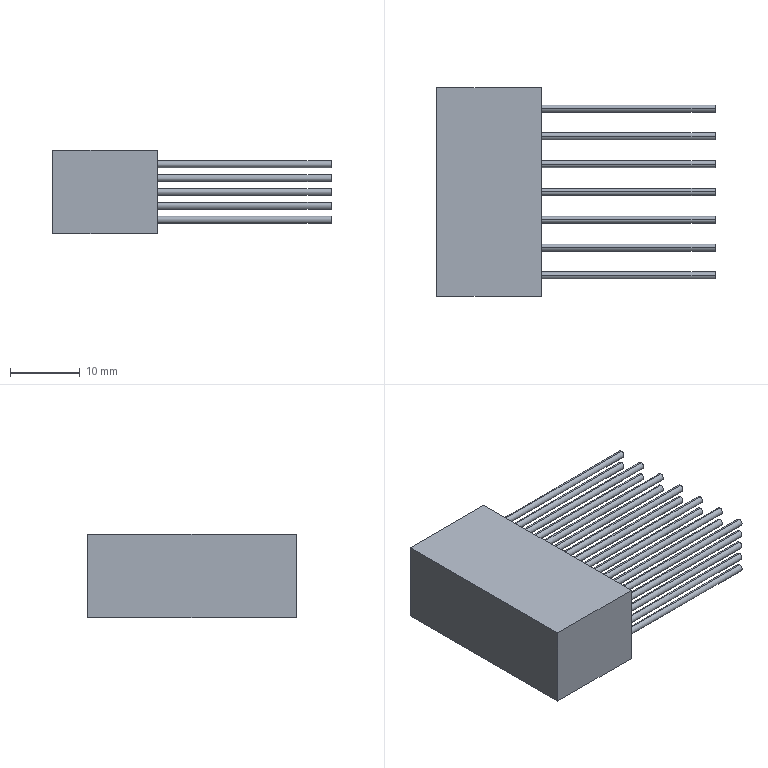Part | SolidWorks | features Extrusion 1, ICE 1, LPattern 1, MirrorPattern 1 | 1 solid | 111 faces | box 40 x 30 x 12 mm | volume 6087 mm3 | cylinder 70 | plane 41 | commonest cylinder face diameters 1 x70